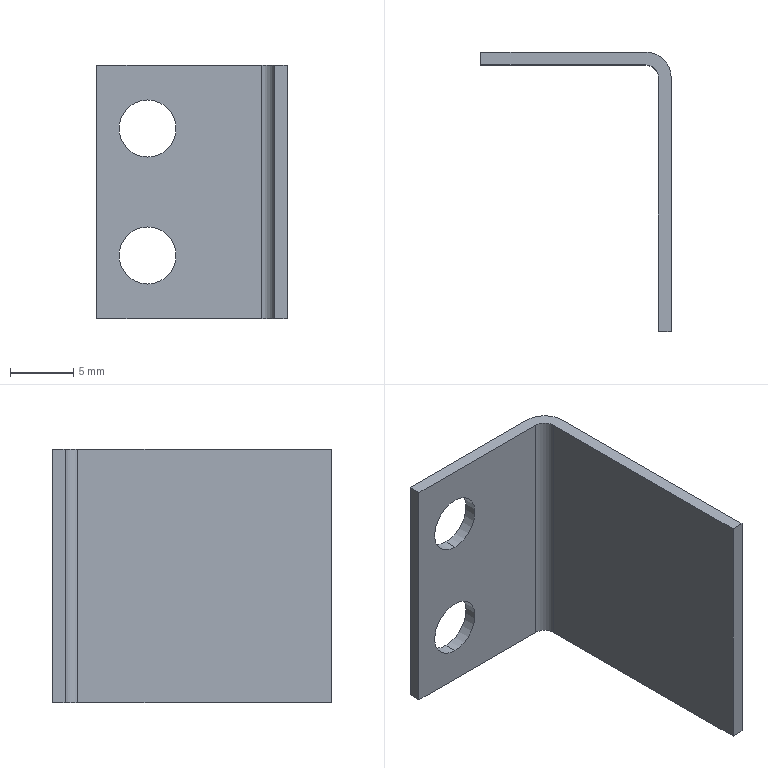Part | STEP file | 0243_222_Dog | 1 solid | 14 faces | box 15 x 22 x 20 mm | volume 675.315 mm3 | plane 8 | cylinder 6 | commonest cylinder face diameters 4.5 x4 2 x1 4 x1
STEP:
#1=CARTESIAN_POINT('',(0.,0.,0.));
#2=DIRECTION('',(0.,0.,1.));
#3=DIRECTION('',(1.,0.,0.));
#4=AXIS2_PLACEMENT_3D('',#1,#2,#3);
#5=CARTESIAN_POINT('',(-11.,-1.,7.25));
#6=VERTEX_POINT('',#5);
#7=CARTESIAN_POINT('',(-11.,0.,7.25));
#8=VERTEX_POINT('',#7);
#9=CARTESIAN_POINT('',(-11.,0.,7.25));
#10=DIRECTION('',(0.,1.,0.));
#11=VECTOR('',#10,1.);
#12=LINE('',#9,#11);
#13=CARTESIAN_POINT('',(-11.,0.,5.));
#14=DIRECTION('',(0.,1.,0.));
#15=DIRECTION('',(0.,0.,1.));
#16=AXIS2_PLACEMENT_3D('',#13,#14,#15);
#17=CYLINDRICAL_SURFACE('',#16,2.25);
#18=CARTESIAN_POINT('',(6.283,0.));
#19=DIRECTION('',(0.,1.));
#20=VECTOR('',#19,1.);
#21=LINE('',#18,#20);
#22=(GEOMETRIC_REPRESENTATION_CONTEXT(2)PARAMETRIC_REPRESENTATION_CONTEXT()REPRESENTATION_CONTEXT('',''));
#23=DEFINITIONAL_REPRESENTATION('',(#21),#22);
#24=PCURVE('',#17,#23);
#25=CARTESIAN_POINT('',(-11.,0.,5.));
#26=DIRECTION('',(0.,1.,0.));
#27=DIRECTION('',(0.,0.,1.));
#28=AXIS2_PLACEMENT_3D('',#25,#26,#27);
#29=CYLINDRICAL_SURFACE('',#28,2.25);
#30=CARTESIAN_POINT('',(0.,0.));
#31=DIRECTION('',(0.,1.));
#32=VECTOR('',#31,1.);
#33=LINE('',#30,#32);
#34=(GEOMETRIC_REPRESENTATION_CONTEXT(2)PARAMETRIC_REPRESENTATION_CONTEXT()REPRESENTATION_CONTEXT('',''));
#35=DEFINITIONAL_REPRESENTATION('',(#33),#34);
#36=PCURVE('',#29,#35);
#37=SURFACE_CURVE('',#12,(#24,#36),.PCURVE_S1.);
#38=EDGE_CURVE('',#6,#8,#37,.T.);
#39=ORIENTED_EDGE('',*,*,#38,.T.);
#40=CARTESIAN_POINT('',(-11.,0.,2.75));
#41=VERTEX_POINT('',#40);
#42=CARTESIAN_POINT('',(-11.,0.,5.));
#43=DIRECTION('',(0.,1.,0.));
#44=DIRECTION('',(0.,0.,1.));
#45=AXIS2_PLACEMENT_3D('',#42,#43,#44);
#46=CIRCLE('',#45,2.25);
#47=CARTESIAN_POINT('',(0.,0.));
#48=DIRECTION('',(1.,0.));
#49=VECTOR('',#48,1.);
#50=LINE('',#47,#49);
#51=(GEOMETRIC_REPRESENTATION_CONTEXT(2)PARAMETRIC_REPRESENTATION_CONTEXT()REPRESENTATION_CONTEXT('',''));
#52=DEFINITIONAL_REPRESENTATION('',(#50),#51);
#53=PCURVE('',#17,#52);
#54=CARTESIAN_POINT('',(-15.,0.,10.));
#55=DIRECTION('',(0.,-1.,0.));
#56=DIRECTION('',(0.,0.,-1.));
#57=AXIS2_PLACEMENT_3D('',#54,#55,#56);
#58=PLANE('',#57);
#59=CARTESIAN_POINT('',(2.75,4.));
#60=CARTESIAN_POINT('',(2.75,7.897));
#61=CARTESIAN_POINT('',(6.125,5.949));
#62=CARTESIAN_POINT('',(9.5,4.));
#63=CARTESIAN_POINT('',(6.125,2.051));
#64=CARTESIAN_POINT('',(2.75,0.1029));
#65=CARTESIAN_POINT('',(2.75,4.));
#66=(BOUNDED_CURVE()B_SPLINE_CURVE(2,(#59,#60,#61,#62,#63,#64,#65),.UNSPECIFIED.,.T.,.F.)B_SPLINE_CURVE_WITH_KNOTS((1,2,2,2,2,1),(-2.094,0.,2.094,4.189,6.283,8.378),.UNSPECIFIED.)CURVE()GEOMETRIC_REPRESENTATION_ITEM()RATIONAL_B_SPLINE_CURVE((1.,0.5,1.,0.5,1.,0.5,1.))REPRESENTATION_ITEM(''));
#67=(GEOMETRIC_REPRESENTATION_CONTEXT(2)PARAMETRIC_REPRESENTATION_CONTEXT()REPRESENTATION_CONTEXT('',''));
#68=DEFINITIONAL_REPRESENTATION('',(#66),#67);
#69=PCURVE('',#58,#68);
#70=SURFACE_CURVE('',#46,(#53,#69),.PCURVE_S1.);
#71=EDGE_CURVE('',#41,#8,#70,.T.);
#72=ORIENTED_EDGE('',*,*,#71,.F.);
#73=CARTESIAN_POINT('',(-11.,-1.,2.75));
#74=VERTEX_POINT('',#73);
#75=CARTESIAN_POINT('',(-11.,0.,2.75));
#76=DIRECTION('',(0.,1.,0.));
#77=VECTOR('',#76,1.);
#78=LINE('',#75,#77);
#79=CARTESIAN_POINT('',(3.142,0.));
#80=DIRECTION('',(0.,1.));
#81=VECTOR('',#80,1.);
#82=LINE('',#79,#81);
#83=(GEOMETRIC_REPRESENTATION_CONTEXT(2)PARAMETRIC_REPRESENTATION_CONTEXT()REPRESENTATION_CONTEXT('',''));
#84=DEFINITIONAL_REPRESENTATION('',(#82),#83);
#85=PCURVE('',#17,#84);
#86=CARTESIAN_POINT('',(3.142,0.));
#87=DIRECTION('',(0.,1.));
#88=VECTOR('',#87,1.);
#89=LINE('',#86,#88);
#90=(GEOMETRIC_REPRESENTATION_CONTEXT(2)PARAMETRIC_REPRESENTATION_CONTEXT()REPRESENTATION_CONTEXT('',''));
#91=DEFINITIONAL_REPRESENTATION('',(#89),#90);
#92=PCURVE('',#29,#91);
#93=SURFACE_CURVE('',#78,(#85,#92),.PCURVE_S1.);
#94=EDGE_CURVE('',#74,#41,#93,.T.);
#95=ORIENTED_EDGE('',*,*,#94,.F.);
#96=CARTESIAN_POINT('',(-11.,-1.,5.));
#97=DIRECTION('',(0.,1.,0.));
#98=DIRECTION('',(-1.,0.,0.));
#99=AXIS2_PLACEMENT_3D('',#96,#97,#98);
#100=CIRCLE('',#99,2.25);
#101=CARTESIAN_POINT('',(-1.571,-1.));
#102=DIRECTION('',(1.,0.));
#103=VECTOR('',#102,1.);
#104=LINE('',#101,#103);
#105=(GEOMETRIC_REPRESENTATION_CONTEXT(2)PARAMETRIC_REPRESENTATION_CONTEXT()REPRESENTATION_CONTEXT('',''));
#106=DEFINITIONAL_REPRESENTATION('',(#104),#105);
#107=PCURVE('',#17,#106);
#108=CARTESIAN_POINT('',(-15.,-1.,10.));
#109=DIRECTION('',(0.,1.,0.));
#110=DIRECTION('',(-1.,0.,0.));
#111=AXIS2_PLACEMENT_3D('',#108,#109,#110);
#112=PLANE('',#111);
#113=CARTESIAN_POINT('',(-4.,-5.));
#114=DIRECTION('',(1.,0.));
#115=AXIS2_PLACEMENT_2D('',#113,#114);
#116=CIRCLE('',#115,2.25);
#117=(GEOMETRIC_REPRESENTATION_CONTEXT(2)PARAMETRIC_REPRESENTATION_CONTEXT()REPRESENTATION_CONTEXT('',''));
#118=DEFINITIONAL_REPRESENTATION('',(#116),#117);
#119=PCURVE('',#112,#118);
#120=SURFACE_CURVE('',#100,(#107,#119),.PCURVE_S1.);
#121=EDGE_CURVE('',#74,#6,#120,.T.);
#122=ORIENTED_EDGE('',*,*,#121,.T.);
#123=EDGE_LOOP('',(#39,#72,#95,#122));
#124=FACE_BOUND('',#123,.F.);
#125=ADVANCED_FACE('',(#124),#17,.F.);
#126=CARTESIAN_POINT('',(-11.,-1.,-2.75));
#127=VERTEX_POINT('',#126);
#128=CARTESIAN_POINT('',(-11.,0.,-2.75));
#129=VERTEX_POINT('',#128);
#130=CARTESIAN_POINT('',(-11.,0.,-2.75));
#131=DIRECTION('',(0.,1.,0.));
#132=VECTOR('',#131,1.);
#133=LINE('',#130,#132);
#134=CARTESIAN_POINT('',(-11.,0.,-5.));
#135=DIRECTION('',(0.,1.,0.));
#136=DIRECTION('',(0.,0.,1.));
#137=AXIS2_PLACEMENT_3D('',#134,#135,#136);
#138=CYLINDRICAL_SURFACE('',#137,2.25);
#139=CARTESIAN_POINT('',(6.283,0.));
#140=DIRECTION('',(0.,1.));
#141=VECTOR('',#140,1.);
#142=LINE('',#139,#141);
#143=(GEOMETRIC_REPRESENTATION_CONTEXT(2)PARAMETRIC_REPRESENTATION_CONTEXT()REPRESENTATION_CONTEXT('',''));
#144=DEFINITIONAL_REPRESENTATION('',(#142),#143);
#145=PCURVE('',#138,#144);
#146=CARTESIAN_POINT('',(-11.,0.,-5.));
#147=DIRECTION('',(0.,1.,0.));
#148=DIRECTION('',(0.,0.,1.));
#149=AXIS2_PLACEMENT_3D('',#146,#147,#148);
#150=CYLINDRICAL_SURFACE('',#149,2.25);
#151=CARTESIAN_POINT('',(0.,0.));
#152=DIRECTION('',(0.,1.));
#153=VECTOR('',#152,1.);
#154=LINE('',#151,#153);
#155=(GEOMETRIC_REPRESENTATION_CONTEXT(2)PARAMETRIC_REPRESENTATION_CONTEXT()REPRESENTATION_CONTEXT('',''));
#156=DEFINITIONAL_REPRESENTATION('',(#154),#155);
#157=PCURVE('',#150,#156);
#158=SURFACE_CURVE('',#133,(#145,#157),.PCURVE_S1.);
#159=EDGE_CURVE('',#127,#129,#158,.T.);
#160=ORIENTED_EDGE('',*,*,#159,.T.);
#161=CARTESIAN_POINT('',(-11.,0.,-7.25));
#162=VERTEX_POINT('',#161);
#163=CARTESIAN_POINT('',(-11.,0.,-5.));
#164=DIRECTION('',(0.,1.,0.));
#165=DIRECTION('',(0.,0.,1.));
#166=AXIS2_PLACEMENT_3D('',#163,#164,#165);
#167=CIRCLE('',#166,2.25);
#168=CARTESIAN_POINT('',(0.,0.));
#169=DIRECTION('',(1.,0.));
#170=VECTOR('',#169,1.);
#171=LINE('',#168,#170);
#172=(GEOMETRIC_REPRESENTATION_CONTEXT(2)PARAMETRIC_REPRESENTATION_CONTEXT()REPRESENTATION_CONTEXT('',''));
#173=DEFINITIONAL_REPRESENTATION('',(#171),#172);
#174=PCURVE('',#138,#173);
#175=CARTESIAN_POINT('',(12.75,4.));
#176=CARTESIAN_POINT('',(12.75,7.897));
#177=CARTESIAN_POINT('',(16.125,5.949));
#178=CARTESIAN_POINT('',(19.5,4.));
#179=CARTESIAN_POINT('',(16.125,2.051));
#180=CARTESIAN_POINT('',(12.75,0.1029));
#181=CARTESIAN_POINT('',(12.75,4.));
#182=(BOUNDED_CURVE()B_SPLINE_CURVE(2,(#175,#176,#177,#178,#179,#180,#181),.UNSPECIFIED.,.T.,.F.)B_SPLINE_CURVE_WITH_KNOTS((1,2,2,2,2,1),(-2.094,0.,2.094,4.189,6.283,8.378),.UNSPECIFIED.)CURVE()GEOMETRIC_REPRESENTATION_ITEM()RATIONAL_B_SPLINE_CURVE((1.,0.5,1.,0.5,1.,0.5,1.))REPRESENTATION_ITEM(''));
#183=(GEOMETRIC_REPRESENTATION_CONTEXT(2)PARAMETRIC_REPRESENTATION_CONTEXT()REPRESENTATION_CONTEXT('',''));
#184=DEFINITIONAL_REPRESENTATION('',(#182),#183);
#185=PCURVE('',#58,#184);
#186=SURFACE_CURVE('',#167,(#174,#185),.PCURVE_S1.);
#187=EDGE_CURVE('',#162,#129,#186,.T.);
#188=ORIENTED_EDGE('',*,*,#187,.F.);
#189=CARTESIAN_POINT('',(-11.,-1.,-7.25));
#190=VERTEX_POINT('',#189);
#191=CARTESIAN_POINT('',(-11.,0.,-7.25));
#192=DIRECTION('',(0.,1.,0.));
#193=VECTOR('',#192,1.);
#194=LINE('',#191,#193);
#195=CARTESIAN_POINT('',(3.142,0.));
#196=DIRECTION('',(0.,1.));
#197=VECTOR('',#196,1.);
#198=LINE('',#195,#197);
#199=(GEOMETRIC_REPRESENTATION_CONTEXT(2)PARAMETRIC_REPRESENTATION_CONTEXT()REPRESENTATION_CONTEXT('',''));
#200=DEFINITIONAL_REPRESENTATION('',(#198),#199);
#201=PCURVE('',#138,#200);
#202=CARTESIAN_POINT('',(3.142,0.));
#203=DIRECTION('',(0.,1.));
#204=VECTOR('',#203,1.);
#205=LINE('',#202,#204);
#206=(GEOMETRIC_REPRESENTATION_CONTEXT(2)PARAMETRIC_REPRESENTATION_CONTEXT()REPRESENTATION_CONTEXT('',''));
#207=DEFINITIONAL_REPRESENTATION('',(#205),#206);
#208=PCURVE('',#150,#207);
#209=SURFACE_CURVE('',#194,(#201,#208),.PCURVE_S1.);
#210=EDGE_CURVE('',#190,#162,#209,.T.);
#211=ORIENTED_EDGE('',*,*,#210,.F.);
#212=CARTESIAN_POINT('',(-11.,-1.,-5.));
#213=DIRECTION('',(0.,1.,0.));
#214=DIRECTION('',(-1.,0.,0.));
#215=AXIS2_PLACEMENT_3D('',#212,#213,#214);
#216=CIRCLE('',#215,2.25);
#217=CARTESIAN_POINT('',(-1.571,-1.));
#218=DIRECTION('',(1.,0.));
#219=VECTOR('',#218,1.);
#220=LINE('',#217,#219);
#221=(GEOMETRIC_REPRESENTATION_CONTEXT(2)PARAMETRIC_REPRESENTATION_CONTEXT()REPRESENTATION_CONTEXT('',''));
#222=DEFINITIONAL_REPRESENTATION('',(#220),#221);
#223=PCURVE('',#138,#222);
#224=CARTESIAN_POINT('',(-4.,-15.));
#225=DIRECTION('',(1.,0.));
#226=AXIS2_PLACEMENT_2D('',#224,#225);
#227=CIRCLE('',#226,2.25);
#228=(GEOMETRIC_REPRESENTATION_CONTEXT(2)PARAMETRIC_REPRESENTATION_CONTEXT()REPRESENTATION_CONTEXT('',''));
#229=DEFINITIONAL_REPRESENTATION('',(#227),#228);
#230=PCURVE('',#112,#229);
#231=SURFACE_CURVE('',#216,(#223,#230),.PCURVE_S1.);
#232=EDGE_CURVE('',#190,#127,#231,.T.);
#233=ORIENTED_EDGE('',*,*,#232,.T.);
#234=EDGE_LOOP('',(#160,#188,#211,#233));
#235=FACE_BOUND('',#234,.F.);
#236=ADVANCED_FACE('',(#235),#138,.F.);
#237=CARTESIAN_POINT('',(-15.,0.,-10.));
#238=VERTEX_POINT('',#237);
#239=CARTESIAN_POINT('',(-15.,-1.,-10.));
#240=VERTEX_POINT('',#239);
#241=CARTESIAN_POINT('',(-15.,0.,-10.));
#242=DIRECTION('',(0.,-1.,0.));
#243=VECTOR('',#242,1.);
#244=LINE('',#241,#243);
#245=CARTESIAN_POINT('',(-15.,0.,10.));
#246=DIRECTION('',(1.,0.,0.));
#247=DIRECTION('',(0.,0.,-1.));
#248=AXIS2_PLACEMENT_3D('',#245,#246,#247);
#249=PLANE('',#248);
#250=CARTESIAN_POINT('',(20.,0.));
#251=DIRECTION('',(0.,-1.));
#252=VECTOR('',#251,1.);
#253=LINE('',#250,#252);
#254=(GEOMETRIC_REPRESENTATION_CONTEXT(2)PARAMETRIC_REPRESENTATION_CONTEXT()REPRESENTATION_CONTEXT('',''));
#255=DEFINITIONAL_REPRESENTATION('',(#253),#254);
#256=PCURVE('',#249,#255);
#257=CARTESIAN_POINT('',(-15.,-1.,-10.));
#258=DIRECTION('',(0.,0.,1.));
#259=DIRECTION('',(1.,0.,0.));
#260=AXIS2_PLACEMENT_3D('',#257,#258,#259);
#261=PLANE('',#260);
#262=CARTESIAN_POINT('',(0.,1.));
#263=DIRECTION('',(0.,-1.));
#264=VECTOR('',#263,1.);
#265=LINE('',#262,#264);
#266=(GEOMETRIC_REPRESENTATION_CONTEXT(2)PARAMETRIC_REPRESENTATION_CONTEXT()REPRESENTATION_CONTEXT('',''));
#267=DEFINITIONAL_REPRESENTATION('',(#265),#266);
#268=PCURVE('',#261,#267);
#269=SURFACE_CURVE('',#244,(#256,#268),.PCURVE_S1.);
#270=EDGE_CURVE('',#238,#240,#269,.T.);
#271=ORIENTED_EDGE('',*,*,#270,.T.);
#272=CARTESIAN_POINT('',(-15.,-1.,10.));
#273=VERTEX_POINT('',#272);
#274=CARTESIAN_POINT('',(-15.,-1.,10.));
#275=DIRECTION('',(0.,0.,-1.));
#276=VECTOR('',#275,1.);
#277=LINE('',#274,#276);
#278=CARTESIAN_POINT('',(0.,-1.));
#279=DIRECTION('',(1.,0.));
#280=VECTOR('',#279,1.);
#281=LINE('',#278,#280);
#282=(GEOMETRIC_REPRESENTATION_CONTEXT(2)PARAMETRIC_REPRESENTATION_CONTEXT()REPRESENTATION_CONTEXT('',''));
#283=DEFINITIONAL_REPRESENTATION('',(#281),#282);
#284=PCURVE('',#249,#283);
#285=CARTESIAN_POINT('',(0.,0.));
#286=DIRECTION('',(0.,-1.));
#287=VECTOR('',#286,1.);
#288=LINE('',#285,#287);
#289=(GEOMETRIC_REPRESENTATION_CONTEXT(2)PARAMETRIC_REPRESENTATION_CONTEXT()REPRESENTATION_CONTEXT('',''));
#290=DEFINITIONAL_REPRESENTATION('',(#288),#289);
#291=PCURVE('',#112,#290);
#292=SURFACE_CURVE('',#277,(#284,#291),.PCURVE_S1.);
#293=EDGE_CURVE('',#273,#240,#292,.T.);
#294=ORIENTED_EDGE('',*,*,#293,.F.);
#295=CARTESIAN_POINT('',(-15.,0.,10.));
#296=VERTEX_POINT('',#295);
#297=CARTESIAN_POINT('',(-15.,0.,10.));
#298=DIRECTION('',(0.,-1.,0.));
#299=VECTOR('',#298,1.);
#300=LINE('',#297,#299);
#301=CARTESIAN_POINT('',(0.,0.));
#302=DIRECTION('',(0.,-1.));
#303=VECTOR('',#302,1.);
#304=LINE('',#301,#303);
#305=(GEOMETRIC_REPRESENTATION_CONTEXT(2)PARAMETRIC_REPRESENTATION_CONTEXT()REPRESENTATION_CONTEXT('',''));
#306=DEFINITIONAL_REPRESENTATION('',(#304),#305);
#307=PCURVE('',#249,#306);
#308=CARTESIAN_POINT('',(-15.,-1.,10.));
#309=DIRECTION('',(0.,0.,1.));
#310=DIRECTION('',(1.,0.,0.));
#311=AXIS2_PLACEMENT_3D('',#308,#309,#310);
#312=PLANE('',#311);
#313=CARTESIAN_POINT('',(0.,1.));
#314=DIRECTION('',(0.,-1.));
#315=VECTOR('',#314,1.);
#316=LINE('',#313,#315);
#317=(GEOMETRIC_REPRESENTATION_CONTEXT(2)PARAMETRIC_REPRESENTATION_CONTEXT()REPRESENTATION_CONTEXT('',''));
#318=DEFINITIONAL_REPRESENTATION('',(#316),#317);
#319=PCURVE('',#312,#318);
#320=SURFACE_CURVE('',#300,(#307,#319),.PCURVE_S1.);
#321=EDGE_CURVE('',#296,#273,#320,.T.);
#322=ORIENTED_EDGE('',*,*,#321,.F.);
#323=CARTESIAN_POINT('',(-15.,0.,10.));
#324=DIRECTION('',(0.,0.,-1.));
#325=VECTOR('',#324,1.);
#326=LINE('',#323,#325);
#327=CARTESIAN_POINT('',(0.,0.));
#328=DIRECTION('',(1.,0.));
#329=VECTOR('',#328,1.);
#330=LINE('',#327,#329);
#331=(GEOMETRIC_REPRESENTATION_CONTEXT(2)PARAMETRIC_REPRESENTATION_CONTEXT()REPRESENTATION_CONTEXT('',''));
#332=DEFINITIONAL_REPRESENTATION('',(#330),#331);
#333=PCURVE('',#249,#332);
#334=CARTESIAN_POINT('',(0.,0.));
#335=DIRECTION('',(1.,0.));
#336=VECTOR('',#335,1.);
#337=LINE('',#334,#336);
#338=(GEOMETRIC_REPRESENTATION_CONTEXT(2)PARAMETRIC_REPRESENTATION_CONTEXT()REPRESENTATION_CONTEXT('',''));
#339=DEFINITIONAL_REPRESENTATION('',(#337),#338);
#340=PCURVE('',#58,#339);
#341=SURFACE_CURVE('',#326,(#333,#340),.PCURVE_S1.);
#342=EDGE_CURVE('',#296,#238,#341,.T.);
#343=ORIENTED_EDGE('',*,*,#342,.T.);
#344=EDGE_LOOP('',(#271,#294,#322,#343));
#345=FACE_BOUND('',#344,.T.);
#346=ADVANCED_FACE('',(#345),#249,.F.);
#347=CARTESIAN_POINT('',(-11.,-1.,5.));
#348=DIRECTION('',(0.,1.,0.));
#349=DIRECTION('',(-1.,0.,0.));
#350=AXIS2_PLACEMENT_3D('',#347,#348,#349);
#351=CIRCLE('',#350,2.25);
#352=CARTESIAN_POINT('',(-4.,-5.));
#353=DIRECTION('',(1.,0.));
#354=AXIS2_PLACEMENT_2D('',#352,#353);
#355=CIRCLE('',#354,2.25);
#356=(GEOMETRIC_REPRESENTATION_CONTEXT(2)PARAMETRIC_REPRESENTATION_CONTEXT()REPRESENTATION_CONTEXT('',''));
#357=DEFINITIONAL_REPRESENTATION('',(#355),#356);
#358=PCURVE('',#112,#357);
#359=CARTESIAN_POINT('',(-1.571,-1.));
#360=DIRECTION('',(1.,0.));
#361=VECTOR('',#360,1.);
#362=LINE('',#359,#361);
#363=(GEOMETRIC_REPRESENTATION_CONTEXT(2)PARAMETRIC_REPRESENTATION_CONTEXT()REPRESENTATION_CONTEXT('',''));
#364=DEFINITIONAL_REPRESENTATION('',(#362),#363);
#365=PCURVE('',#29,#364);
#366=SURFACE_CURVE('',#351,(#358,#365),.PCURVE_S1.);
#367=EDGE_CURVE('',#6,#74,#366,.T.);
#368=ORIENTED_EDGE('',*,*,#367,.T.);
#369=ORIENTED_EDGE('',*,*,#121,.T.);
#370=EDGE_LOOP('',(#368,#369));
#371=FACE_BOUND('',#370,.T.);
#372=CARTESIAN_POINT('',(-11.,-1.,-5.));
#373=DIRECTION('',(0.,1.,0.));
#374=DIRECTION('',(-1.,0.,0.));
#375=AXIS2_PLACEMENT_3D('',#372,#373,#374);
#376=CIRCLE('',#375,2.25);
#377=CARTESIAN_POINT('',(-4.,-15.));
#378=DIRECTION('',(1.,0.));
#379=AXIS2_PLACEMENT_2D('',#377,#378);
#380=CIRCLE('',#379,2.25);
#381=(GEOMETRIC_REPRESENTATION_CONTEXT(2)PARAMETRIC_REPRESENTATION_CONTEXT()REPRESENTATION_CONTEXT('',''));
#382=DEFINITIONAL_REPRESENTATION('',(#380),#381);
#383=PCURVE('',#112,#382);
#384=CARTESIAN_POINT('',(-1.571,-1.));
#385=DIRECTION('',(1.,0.));
#386=VECTOR('',#385,1.);
#387=LINE('',#384,#386);
#388=(GEOMETRIC_REPRESENTATION_CONTEXT(2)PARAMETRIC_REPRESENTATION_CONTEXT()REPRESENTATION_CONTEXT('',''));
#389=DEFINITIONAL_REPRESENTATION('',(#387),#388);
#390=PCURVE('',#150,#389);
#391=SURFACE_CURVE('',#376,(#383,#390),.PCURVE_S1.);
#392=EDGE_CURVE('',#127,#190,#391,.T.);
#393=ORIENTED_EDGE('',*,*,#392,.T.);
#394=ORIENTED_EDGE('',*,*,#232,.T.);
#395=EDGE_LOOP('',(#393,#394));
#396=FACE_BOUND('',#395,.T.);
#397=CARTESIAN_POINT('',(-2.,-1.,-10.));
#398=VERTEX_POINT('',#397);
#399=CARTESIAN_POINT('',(-15.,-1.,-10.));
#400=DIRECTION('',(1.,0.,0.));
#401=VECTOR('',#400,1.);
#402=LINE('',#399,#401);
#403=CARTESIAN_POINT('',(0.,-20.));
#404=DIRECTION('',(-1.,0.));
#405=VECTOR('',#404,1.);
#406=LINE('',#403,#405);
#407=(GEOMETRIC_REPRESENTATION_CONTEXT(2)PARAMETRIC_REPRESENTATION_CONTEXT()REPRESENTATION_CONTEXT('',''));
#408=DEFINITIONAL_REPRESENTATION('',(#406),#407);
#409=PCURVE('',#112,#408);
#410=CARTESIAN_POINT('',(0.,0.));
#411=DIRECTION('',(1.,0.));
#412=VECTOR('',#411,1.);
#413=LINE('',#410,#412);
#414=(GEOMETRIC_REPRESENTATION_CONTEXT(2)PARAMETRIC_REPRESENTATION_CONTEXT()REPRESENTATION_CONTEXT('',''));
#415=DEFINITIONAL_REPRESENTATION('',(#413),#414);
#416=PCURVE('',#261,#415);
#417=SURFACE_CURVE('',#402,(#409,#416),.PCURVE_S1.);
#418=EDGE_CURVE('',#240,#398,#417,.T.);
#419=ORIENTED_EDGE('',*,*,#418,.T.);
#420=CARTESIAN_POINT('',(-2.,-1.,10.));
#421=VERTEX_POINT('',#420);
#422=CARTESIAN_POINT('',(-2.,-1.,10.));
#423=DIRECTION('',(0.,0.,1.));
#424=VECTOR('',#423,1.);
#425=LINE('',#422,#424);
#426=CARTESIAN_POINT('',(-13.,0.));
#427=DIRECTION('',(0.,1.));
#428=VECTOR('',#427,1.);
#429=LINE('',#426,#428);
#430=(GEOMETRIC_REPRESENTATION_CONTEXT(2)PARAMETRIC_REPRESENTATION_CONTEXT()REPRESENTATION_CONTEXT('',''));
#431=DEFINITIONAL_REPRESENTATION('',(#429),#430);
#432=PCURVE('',#112,#431);
#433=CARTESIAN_POINT('',(-2.,-2.,10.));
#434=DIRECTION('',(0.,0.,1.));
#435=DIRECTION('',(1.,0.,0.));
#436=AXIS2_PLACEMENT_3D('',#433,#434,#435);
#437=CYLINDRICAL_SURFACE('',#436,1.);
#438=CARTESIAN_POINT('',(1.571,0.));
#439=DIRECTION('',(0.,1.));
#440=VECTOR('',#439,1.);
#441=LINE('',#438,#440);
#442=(GEOMETRIC_REPRESENTATION_CONTEXT(2)PARAMETRIC_REPRESENTATION_CONTEXT()REPRESENTATION_CONTEXT('',''));
#443=DEFINITIONAL_REPRESENTATION('',(#441),#442);
#444=PCURVE('',#437,#443);
#445=SURFACE_CURVE('',#425,(#432,#444),.PCURVE_S1.);
#446=EDGE_CURVE('',#398,#421,#445,.T.);
#447=ORIENTED_EDGE('',*,*,#446,.T.);
#448=CARTESIAN_POINT('',(-15.,-1.,10.));
#449=DIRECTION('',(1.,0.,0.));
#450=VECTOR('',#449,1.);
#451=LINE('',#448,#450);
#452=CARTESIAN_POINT('',(0.,0.));
#453=DIRECTION('',(-1.,0.));
#454=VECTOR('',#453,1.);
#455=LINE('',#452,#454);
#456=(GEOMETRIC_REPRESENTATION_CONTEXT(2)PARAMETRIC_REPRESENTATION_CONTEXT()REPRESENTATION_CONTEXT('',''));
#457=DEFINITIONAL_REPRESENTATION('',(#455),#456);
#458=PCURVE('',#112,#457);
#459=CARTESIAN_POINT('',(0.,0.));
#460=DIRECTION('',(1.,0.));
#461=VECTOR('',#460,1.);
#462=LINE('',#459,#461);
#463=(GEOMETRIC_REPRESENTATION_CONTEXT(2)PARAMETRIC_REPRESENTATION_CONTEXT()REPRESENTATION_CONTEXT('',''));
#464=DEFINITIONAL_REPRESENTATION('',(#462),#463);
#465=PCURVE('',#312,#464);
#466=SURFACE_CURVE('',#451,(#458,#465),.PCURVE_S1.);
#467=EDGE_CURVE('',#273,#421,#466,.T.);
#468=ORIENTED_EDGE('',*,*,#467,.F.);
#469=ORIENTED_EDGE('',*,*,#293,.T.);
#470=EDGE_LOOP('',(#419,#447,#468,#469));
#471=FACE_BOUND('',#470,.T.);
#472=ADVANCED_FACE('',(#371,#396,#471),#112,.F.);
#473=CARTESIAN_POINT('',(-1.,-2.,10.));
#474=VERTEX_POINT('',#473);
#475=CARTESIAN_POINT('',(-1.,-22.,10.));
#476=VERTEX_POINT('',#475);
#477=CARTESIAN_POINT('',(-1.,-1.,10.));
#478=DIRECTION('',(0.,-1.,0.));
#479=VECTOR('',#478,1.);
#480=LINE('',#477,#479);
#481=CARTESIAN_POINT('',(-1.,-1.,10.));
#482=DIRECTION('',(1.,0.,0.));
#483=DIRECTION('',(0.,1.,0.));
#484=AXIS2_PLACEMENT_3D('',#481,#482,#483);
#485=PLANE('',#484);
#486=CARTESIAN_POINT('',(0.,0.));
#487=DIRECTION('',(-1.,0.));
#488=VECTOR('',#487,1.);
#489=LINE('',#486,#488);
#490=(GEOMETRIC_REPRESENTATION_CONTEXT(2)PARAMETRIC_REPRESENTATION_CONTEXT()REPRESENTATION_CONTEXT('',''));
#491=DEFINITIONAL_REPRESENTATION('',(#489),#490);
#492=PCURVE('',#485,#491);
#493=CARTESIAN_POINT('',(14.,0.));
#494=DIRECTION('',(0.,-1.));
#495=VECTOR('',#494,1.);
#496=LINE('',#493,#495);
#497=(GEOMETRIC_REPRESENTATION_CONTEXT(2)PARAMETRIC_REPRESENTATION_CONTEXT()REPRESENTATION_CONTEXT('',''));
#498=DEFINITIONAL_REPRESENTATION('',(#496),#497);
#499=PCURVE('',#312,#498);
#500=SURFACE_CURVE('',#480,(#492,#499),.PCURVE_S1.);
#501=EDGE_CURVE('',#474,#476,#500,.T.);
#502=ORIENTED_EDGE('',*,*,#501,.F.);
#503=CARTESIAN_POINT('',(-1.,-2.,-10.));
#504=VERTEX_POINT('',#503);
#505=CARTESIAN_POINT('',(-1.,-2.,-10.));
#506=DIRECTION('',(0.,0.,-1.));
#507=VECTOR('',#506,1.);
#508=LINE('',#505,#507);
#509=CARTESIAN_POINT('',(-1.,-20.));
#510=DIRECTION('',(0.,-1.));
#511=VECTOR('',#510,1.);
#512=LINE('',#509,#511);
#513=(GEOMETRIC_REPRESENTATION_CONTEXT(2)PARAMETRIC_REPRESENTATION_CONTEXT()REPRESENTATION_CONTEXT('',''));
#514=DEFINITIONAL_REPRESENTATION('',(#512),#513);
#515=PCURVE('',#485,#514);
#516=CARTESIAN_POINT('',(0.,-20.));
#517=DIRECTION('',(0.,-1.));
#518=VECTOR('',#517,1.);
#519=LINE('',#516,#518);
#520=(GEOMETRIC_REPRESENTATION_CONTEXT(2)PARAMETRIC_REPRESENTATION_CONTEXT()REPRESENTATION_CONTEXT('',''));
#521=DEFINITIONAL_REPRESENTATION('',(#519),#520);
#522=PCURVE('',#437,#521);
#523=SURFACE_CURVE('',#508,(#515,#522),.PCURVE_S1.);
#524=EDGE_CURVE('',#474,#504,#523,.T.);
#525=ORIENTED_EDGE('',*,*,#524,.T.);
#526=CARTESIAN_POINT('',(-1.,-22.,-10.));
#527=VERTEX_POINT('',#526);
#528=CARTESIAN_POINT('',(-1.,-1.,-10.));
#529=DIRECTION('',(0.,-1.,0.));
#530=VECTOR('',#529,1.);
#531=LINE('',#528,#530);
#532=CARTESIAN_POINT('',(0.,-20.));
#533=DIRECTION('',(-1.,0.));
#534=VECTOR('',#533,1.);
#535=LINE('',#532,#534);
#536=(GEOMETRIC_REPRESENTATION_CONTEXT(2)PARAMETRIC_REPRESENTATION_CONTEXT()REPRESENTATION_CONTEXT('',''));
#537=DEFINITIONAL_REPRESENTATION('',(#535),#536);
#538=PCURVE('',#485,#537);
#539=CARTESIAN_POINT('',(14.,0.));
#540=DIRECTION('',(0.,-1.));
#541=VECTOR('',#540,1.);
#542=LINE('',#539,#541);
#543=(GEOMETRIC_REPRESENTATION_CONTEXT(2)PARAMETRIC_REPRESENTATION_CONTEXT()REPRESENTATION_CONTEXT('',''));
#544=DEFINITIONAL_REPRESENTATION('',(#542),#543);
#545=PCURVE('',#261,#544);
#546=SURFACE_CURVE('',#531,(#538,#545),.PCURVE_S1.);
#547=EDGE_CURVE('',#504,#527,#546,.T.);
#548=ORIENTED_EDGE('',*,*,#547,.T.);
#549=CARTESIAN_POINT('',(-1.,-22.,10.));
#550=DIRECTION('',(0.,0.,-1.));
#551=VECTOR('',#550,1.);
#552=LINE('',#549,#551);
#553=CARTESIAN_POINT('',(-21.,0.));
#554=DIRECTION('',(0.,-1.));
#555=VECTOR('',#554,1.);
#556=LINE('',#553,#555);
#557=(GEOMETRIC_REPRESENTATION_CONTEXT(2)PARAMETRIC_REPRESENTATION_CONTEXT()REPRESENTATION_CONTEXT('',''));
#558=DEFINITIONAL_REPRESENTATION('',(#556),#557);
#559=PCURVE('',#485,#558);
#560=CARTESIAN_POINT('',(0.,-22.,10.));
#561=DIRECTION('',(0.,1.,0.));
#562=DIRECTION('',(0.,0.,1.));
#563=AXIS2_PLACEMENT_3D('',#560,#561,#562);
#564=PLANE('',#563);
#565=CARTESIAN_POINT('',(0.,-1.));
#566=DIRECTION('',(-1.,0.));
#567=VECTOR('',#566,1.);
#568=LINE('',#565,#567);
#569=(GEOMETRIC_REPRESENTATION_CONTEXT(2)PARAMETRIC_REPRESENTATION_CONTEXT()REPRESENTATION_CONTEXT('',''));
#570=DEFINITIONAL_REPRESENTATION('',(#568),#569);
#571=PCURVE('',#564,#570);
#572=SURFACE_CURVE('',#552,(#559,#571),.PCURVE_S1.);
#573=EDGE_CURVE('',#476,#527,#572,.T.);
#574=ORIENTED_EDGE('',*,*,#573,.F.);
#575=EDGE_LOOP('',(#502,#525,#548,#574));
#576=FACE_BOUND('',#575,.T.);
#577=ADVANCED_FACE('',(#576),#485,.F.);
#578=CARTESIAN_POINT('',(0.,-22.,-10.));
#579=VERTEX_POINT('',#578);
#580=CARTESIAN_POINT('',(0.,-22.,-10.));
#581=DIRECTION('',(1.,0.,0.));
#582=VECTOR('',#581,1.);
#583=LINE('',#580,#582);
#584=CARTESIAN_POINT('',(-20.,0.));
#585=DIRECTION('',(0.,1.));
#586=VECTOR('',#585,1.);
#587=LINE('',#584,#586);
#588=(GEOMETRIC_REPRESENTATION_CONTEXT(2)PARAMETRIC_REPRESENTATION_CONTEXT()REPRESENTATION_CONTEXT('',''));
#589=DEFINITIONAL_REPRESENTATION('',(#587),#588);
#590=PCURVE('',#564,#589);
#591=CARTESIAN_POINT('',(15.,-21.));
#592=DIRECTION('',(1.,0.));
#593=VECTOR('',#592,1.);
#594=LINE('',#591,#593);
#595=(GEOMETRIC_REPRESENTATION_CONTEXT(2)PARAMETRIC_REPRESENTATION_CONTEXT()REPRESENTATION_CONTEXT('',''));
#596=DEFINITIONAL_REPRESENTATION('',(#594),#595);
#597=PCURVE('',#261,#596);
#598=SURFACE_CURVE('',#583,(#590,#597),.PCURVE_S1.);
#599=EDGE_CURVE('',#527,#579,#598,.T.);
#600=ORIENTED_EDGE('',*,*,#599,.T.);
#601=CARTESIAN_POINT('',(0.,-22.,10.));
#602=VERTEX_POINT('',#601);
#603=CARTESIAN_POINT('',(0.,-22.,10.));
#604=DIRECTION('',(0.,0.,-1.));
#605=VECTOR('',#604,1.);
#606=LINE('',#603,#605);
#607=CARTESIAN_POINT('',(0.,0.));
#608=DIRECTION('',(-1.,0.));
#609=VECTOR('',#608,1.);
#610=LINE('',#607,#609);
#611=(GEOMETRIC_REPRESENTATION_CONTEXT(2)PARAMETRIC_REPRESENTATION_CONTEXT()REPRESENTATION_CONTEXT('',''));
#612=DEFINITIONAL_REPRESENTATION('',(#610),#611);
#613=PCURVE('',#564,#612);
#614=CARTESIAN_POINT('',(0.,0.,10.));
#615=DIRECTION('',(-1.,0.,0.));
#616=DIRECTION('',(0.,-1.,0.));
#617=AXIS2_PLACEMENT_3D('',#614,#615,#616);
#618=PLANE('',#617);
#619=CARTESIAN_POINT('',(22.,0.));
#620=DIRECTION('',(0.,-1.));
#621=VECTOR('',#620,1.);
#622=LINE('',#619,#621);
#623=(GEOMETRIC_REPRESENTATION_CONTEXT(2)PARAMETRIC_REPRESENTATION_CONTEXT()REPRESENTATION_CONTEXT('',''));
#624=DEFINITIONAL_REPRESENTATION('',(#622),#623);
#625=PCURVE('',#618,#624);
#626=SURFACE_CURVE('',#606,(#613,#625),.PCURVE_S1.);
#627=EDGE_CURVE('',#602,#579,#626,.T.);
#628=ORIENTED_EDGE('',*,*,#627,.F.);
#629=CARTESIAN_POINT('',(0.,-22.,10.));
#630=DIRECTION('',(1.,0.,0.));
#631=VECTOR('',#630,1.);
#632=LINE('',#629,#631);
#633=CARTESIAN_POINT('',(0.,0.));
#634=DIRECTION('',(0.,1.));
#635=VECTOR('',#634,1.);
#636=LINE('',#633,#635);
#637=(GEOMETRIC_REPRESENTATION_CONTEXT(2)PARAMETRIC_REPRESENTATION_CONTEXT()REPRESENTATION_CONTEXT('',''));
#638=DEFINITIONAL_REPRESENTATION('',(#636),#637);
#639=PCURVE('',#564,#638);
#640=CARTESIAN_POINT('',(15.,-21.));
#641=DIRECTION('',(1.,0.));
#642=VECTOR('',#641,1.);
#643=LINE('',#640,#642);
#644=(GEOMETRIC_REPRESENTATION_CONTEXT(2)PARAMETRIC_REPRESENTATION_CONTEXT()REPRESENTATION_CONTEXT('',''));
#645=DEFINITIONAL_REPRESENTATION('',(#643),#644);
#646=PCURVE('',#312,#645);
#647=SURFACE_CURVE('',#632,(#639,#646),.PCURVE_S1.);
#648=EDGE_CURVE('',#476,#602,#647,.T.);
#649=ORIENTED_EDGE('',*,*,#648,.F.);
#650=ORIENTED_EDGE('',*,*,#573,.T.);
#651=EDGE_LOOP('',(#600,#628,#649,#650));
#652=FACE_BOUND('',#651,.T.);
#653=ADVANCED_FACE('',(#652),#564,.F.);
#654=CARTESIAN_POINT('',(0.,-2.,-10.));
#655=VERTEX_POINT('',#654);
#656=CARTESIAN_POINT('',(0.,0.,-10.));
#657=DIRECTION('',(0.,1.,0.));
#658=VECTOR('',#657,1.);
#659=LINE('',#656,#658);
#660=CARTESIAN_POINT('',(0.,-20.));
#661=DIRECTION('',(-1.,0.));
#662=VECTOR('',#661,1.);
#663=LINE('',#660,#662);
#664=(GEOMETRIC_REPRESENTATION_CONTEXT(2)PARAMETRIC_REPRESENTATION_CONTEXT()REPRESENTATION_CONTEXT('',''));
#665=DEFINITIONAL_REPRESENTATION('',(#663),#664);
#666=PCURVE('',#618,#665);
#667=CARTESIAN_POINT('',(15.,1.));
#668=DIRECTION('',(0.,1.));
#669=VECTOR('',#668,1.);
#670=LINE('',#667,#669);
#671=(GEOMETRIC_REPRESENTATION_CONTEXT(2)PARAMETRIC_REPRESENTATION_CONTEXT()REPRESENTATION_CONTEXT('',''));
#672=DEFINITIONAL_REPRESENTATION('',(#670),#671);
#673=PCURVE('',#261,#672);
#674=SURFACE_CURVE('',#659,(#666,#673),.PCURVE_S1.);
#675=EDGE_CURVE('',#579,#655,#674,.T.);
#676=ORIENTED_EDGE('',*,*,#675,.T.);
#677=CARTESIAN_POINT('',(0.,-2.,10.));
#678=VERTEX_POINT('',#677);
#679=CARTESIAN_POINT('',(0.,-2.,10.));
#680=DIRECTION('',(0.,0.,1.));
#681=VECTOR('',#680,1.);
#682=LINE('',#679,#681);
#683=CARTESIAN_POINT('',(2.,0.));
#684=DIRECTION('',(0.,1.));
#685=VECTOR('',#684,1.);
#686=LINE('',#683,#685);
#687=(GEOMETRIC_REPRESENTATION_CONTEXT(2)PARAMETRIC_REPRESENTATION_CONTEXT()REPRESENTATION_CONTEXT('',''));
#688=DEFINITIONAL_REPRESENTATION('',(#686),#687);
#689=PCURVE('',#618,#688);
#690=CARTESIAN_POINT('',(-2.,-2.,10.));
#691=DIRECTION('',(0.,0.,-1.));
#692=DIRECTION('',(-1.,0.,0.));
#693=AXIS2_PLACEMENT_3D('',#690,#691,#692);
#694=CYLINDRICAL_SURFACE('',#693,2.);
#695=CARTESIAN_POINT('',(3.142,0.));
#696=DIRECTION('',(0.,-1.));
#697=VECTOR('',#696,1.);
#698=LINE('',#695,#697);
#699=(GEOMETRIC_REPRESENTATION_CONTEXT(2)PARAMETRIC_REPRESENTATION_CONTEXT()REPRESENTATION_CONTEXT('',''));
#700=DEFINITIONAL_REPRESENTATION('',(#698),#699);
#701=PCURVE('',#694,#700);
#702=SURFACE_CURVE('',#682,(#689,#701),.PCURVE_S1.);
#703=EDGE_CURVE('',#655,#678,#702,.T.);
#704=ORIENTED_EDGE('',*,*,#703,.T.);
#705=CARTESIAN_POINT('',(0.,0.,10.));
#706=DIRECTION('',(0.,1.,0.));
#707=VECTOR('',#706,1.);
#708=LINE('',#705,#707);
#709=CARTESIAN_POINT('',(0.,0.));
#710=DIRECTION('',(-1.,0.));
#711=VECTOR('',#710,1.);
#712=LINE('',#709,#711);
#713=(GEOMETRIC_REPRESENTATION_CONTEXT(2)PARAMETRIC_REPRESENTATION_CONTEXT()REPRESENTATION_CONTEXT('',''));
#714=DEFINITIONAL_REPRESENTATION('',(#712),#713);
#715=PCURVE('',#618,#714);
#716=CARTESIAN_POINT('',(15.,1.));
#717=DIRECTION('',(0.,1.));
#718=VECTOR('',#717,1.);
#719=LINE('',#716,#718);
#720=(GEOMETRIC_REPRESENTATION_CONTEXT(2)PARAMETRIC_REPRESENTATION_CONTEXT()REPRESENTATION_CONTEXT('',''));
#721=DEFINITIONAL_REPRESENTATION('',(#719),#720);
#722=PCURVE('',#312,#721);
#723=SURFACE_CURVE('',#708,(#715,#722),.PCURVE_S1.);
#724=EDGE_CURVE('',#602,#678,#723,.T.);
#725=ORIENTED_EDGE('',*,*,#724,.F.);
#726=ORIENTED_EDGE('',*,*,#627,.T.);
#727=EDGE_LOOP('',(#676,#704,#725,#726));
#728=FACE_BOUND('',#727,.T.);
#729=ADVANCED_FACE('',(#728),#618,.F.);
#730=CARTESIAN_POINT('',(-11.,0.,5.));
#731=DIRECTION('',(0.,1.,0.));
#732=DIRECTION('',(0.,0.,1.));
#733=AXIS2_PLACEMENT_3D('',#730,#731,#732);
#734=CIRCLE('',#733,2.25);
#735=CARTESIAN_POINT('',(2.75,4.));
#736=CARTESIAN_POINT('',(2.75,7.897));
#737=CARTESIAN_POINT('',(6.125,5.949));
#738=CARTESIAN_POINT('',(9.5,4.));
#739=CARTESIAN_POINT('',(6.125,2.051));
#740=CARTESIAN_POINT('',(2.75,0.1029));
#741=CARTESIAN_POINT('',(2.75,4.));
#742=(BOUNDED_CURVE()B_SPLINE_CURVE(2,(#735,#736,#737,#738,#739,#740,#741),.UNSPECIFIED.,.T.,.F.)B_SPLINE_CURVE_WITH_KNOTS((1,2,2,2,2,1),(-2.094,0.,2.094,4.189,6.283,8.378),.UNSPECIFIED.)CURVE()GEOMETRIC_REPRESENTATION_ITEM()RATIONAL_B_SPLINE_CURVE((1.,0.5,1.,0.5,1.,0.5,1.))REPRESENTATION_ITEM(''));
#743=(GEOMETRIC_REPRESENTATION_CONTEXT(2)PARAMETRIC_REPRESENTATION_CONTEXT()REPRESENTATION_CONTEXT('',''));
#744=DEFINITIONAL_REPRESENTATION('',(#742),#743);
#745=PCURVE('',#58,#744);
#746=CARTESIAN_POINT('',(0.,0.));
#747=DIRECTION('',(1.,0.));
#748=VECTOR('',#747,1.);
#749=LINE('',#746,#748);
#750=(GEOMETRIC_REPRESENTATION_CONTEXT(2)PARAMETRIC_REPRESENTATION_CONTEXT()REPRESENTATION_CONTEXT('',''));
#751=DEFINITIONAL_REPRESENTATION('',(#749),#750);
#752=PCURVE('',#29,#751);
#753=SURFACE_CURVE('',#734,(#745,#752),.PCURVE_S1.);
#754=EDGE_CURVE('',#8,#41,#753,.T.);
#755=ORIENTED_EDGE('',*,*,#754,.F.);
#756=ORIENTED_EDGE('',*,*,#71,.F.);
#757=EDGE_LOOP('',(#755,#756));
#758=FACE_BOUND('',#757,.T.);
#759=CARTESIAN_POINT('',(-11.,0.,-5.));
#760=DIRECTION('',(0.,1.,0.));
#761=DIRECTION('',(0.,0.,1.));
#762=AXIS2_PLACEMENT_3D('',#759,#760,#761);
#763=CIRCLE('',#762,2.25);
#764=CARTESIAN_POINT('',(12.75,4.));
#765=CARTESIAN_POINT('',(12.75,7.897));
#766=CARTESIAN_POINT('',(16.125,5.949));
#767=CARTESIAN_POINT('',(19.5,4.));
#768=CARTESIAN_POINT('',(16.125,2.051));
#769=CARTESIAN_POINT('',(12.75,0.1029));
#770=CARTESIAN_POINT('',(12.75,4.));
#771=(BOUNDED_CURVE()B_SPLINE_CURVE(2,(#764,#765,#766,#767,#768,#769,#770),.UNSPECIFIED.,.T.,.F.)B_SPLINE_CURVE_WITH_KNOTS((1,2,2,2,2,1),(-2.094,0.,2.094,4.189,6.283,8.378),.UNSPECIFIED.)CURVE()GEOMETRIC_REPRESENTATION_ITEM()RATIONAL_B_SPLINE_CURVE((1.,0.5,1.,0.5,1.,0.5,1.))REPRESENTATION_ITEM(''));
#772=(GEOMETRIC_REPRESENTATION_CONTEXT(2)PARAMETRIC_REPRESENTATION_CONTEXT()REPRESENTATION_CONTEXT('',''));
#773=DEFINITIONAL_REPRESENTATION('',(#771),#772);
#774=PCURVE('',#58,#773);
#775=CARTESIAN_POINT('',(0.,0.));
#776=DIRECTION('',(1.,0.));
#777=VECTOR('',#776,1.);
#778=LINE('',#775,#777);
#779=(GEOMETRIC_REPRESENTATION_CONTEXT(2)PARAMETRIC_REPRESENTATION_CONTEXT()REPRESENTATION_CONTEXT('',''));
#780=DEFINITIONAL_REPRESENTATION('',(#778),#779);
#781=PCURVE('',#150,#780);
#782=SURFACE_CURVE('',#763,(#774,#781),.PCURVE_S1.);
#783=EDGE_CURVE('',#129,#162,#782,.T.);
#784=ORIENTED_EDGE('',*,*,#783,.F.);
#785=ORIENTED_EDGE('',*,*,#187,.F.);
#786=EDGE_LOOP('',(#784,#785));
#787=FACE_BOUND('',#786,.T.);
#788=CARTESIAN_POINT('',(-2.,0.,10.));
#789=VERTEX_POINT('',#788);
#790=CARTESIAN_POINT('',(-15.,0.,10.));
#791=DIRECTION('',(-1.,0.,0.));
#792=VECTOR('',#791,1.);
#793=LINE('',#790,#792);
#794=CARTESIAN_POINT('',(0.,0.));
#795=DIRECTION('',(0.,-1.));
#796=VECTOR('',#795,1.);
#797=LINE('',#794,#796);
#798=(GEOMETRIC_REPRESENTATION_CONTEXT(2)PARAMETRIC_REPRESENTATION_CONTEXT()REPRESENTATION_CONTEXT('',''));
#799=DEFINITIONAL_REPRESENTATION('',(#797),#798);
#800=PCURVE('',#58,#799);
#801=CARTESIAN_POINT('',(0.,1.));
#802=DIRECTION('',(-1.,0.));
#803=VECTOR('',#802,1.);
#804=LINE('',#801,#803);
#805=(GEOMETRIC_REPRESENTATION_CONTEXT(2)PARAMETRIC_REPRESENTATION_CONTEXT()REPRESENTATION_CONTEXT('',''));
#806=DEFINITIONAL_REPRESENTATION('',(#804),#805);
#807=PCURVE('',#312,#806);
#808=SURFACE_CURVE('',#793,(#800,#807),.PCURVE_S1.);
#809=EDGE_CURVE('',#789,#296,#808,.T.);
#810=ORIENTED_EDGE('',*,*,#809,.F.);
#811=CARTESIAN_POINT('',(-2.,0.,-10.));
#812=VERTEX_POINT('',#811);
#813=CARTESIAN_POINT('',(-2.,0.,10.));
#814=DIRECTION('',(0.,0.,-1.));
#815=VECTOR('',#814,1.);
#816=LINE('',#813,#815);
#817=CARTESIAN_POINT('',(0.,13.));
#818=DIRECTION('',(1.,0.));
#819=VECTOR('',#818,1.);
#820=LINE('',#817,#819);
#821=(GEOMETRIC_REPRESENTATION_CONTEXT(2)PARAMETRIC_REPRESENTATION_CONTEXT()REPRESENTATION_CONTEXT('',''));
#822=DEFINITIONAL_REPRESENTATION('',(#820),#821);
#823=PCURVE('',#58,#822);
#824=CARTESIAN_POINT('',(1.571,0.));
#825=DIRECTION('',(0.,1.));
#826=VECTOR('',#825,1.);
#827=LINE('',#824,#826);
#828=(GEOMETRIC_REPRESENTATION_CONTEXT(2)PARAMETRIC_REPRESENTATION_CONTEXT()REPRESENTATION_CONTEXT('',''));
#829=DEFINITIONAL_REPRESENTATION('',(#827),#828);
#830=PCURVE('',#694,#829);
#831=SURFACE_CURVE('',#816,(#823,#830),.PCURVE_S1.);
#832=EDGE_CURVE('',#789,#812,#831,.T.);
#833=ORIENTED_EDGE('',*,*,#832,.T.);
#834=CARTESIAN_POINT('',(-15.,0.,-10.));
#835=DIRECTION('',(-1.,0.,0.));
#836=VECTOR('',#835,1.);
#837=LINE('',#834,#836);
#838=CARTESIAN_POINT('',(20.,0.));
#839=DIRECTION('',(0.,-1.));
#840=VECTOR('',#839,1.);
#841=LINE('',#838,#840);
#842=(GEOMETRIC_REPRESENTATION_CONTEXT(2)PARAMETRIC_REPRESENTATION_CONTEXT()REPRESENTATION_CONTEXT('',''));
#843=DEFINITIONAL_REPRESENTATION('',(#841),#842);
#844=PCURVE('',#58,#843);
#845=CARTESIAN_POINT('',(0.,1.));
#846=DIRECTION('',(-1.,0.));
#847=VECTOR('',#846,1.);
#848=LINE('',#845,#847);
#849=(GEOMETRIC_REPRESENTATION_CONTEXT(2)PARAMETRIC_REPRESENTATION_CONTEXT()REPRESENTATION_CONTEXT('',''));
#850=DEFINITIONAL_REPRESENTATION('',(#848),#849);
#851=PCURVE('',#261,#850);
#852=SURFACE_CURVE('',#837,(#844,#851),.PCURVE_S1.);
#853=EDGE_CURVE('',#812,#238,#852,.T.);
#854=ORIENTED_EDGE('',*,*,#853,.T.);
#855=ORIENTED_EDGE('',*,*,#342,.F.);
#856=EDGE_LOOP('',(#810,#833,#854,#855));
#857=FACE_BOUND('',#856,.T.);
#858=ADVANCED_FACE('',(#758,#787,#857),#58,.F.);
#859=ORIENTED_EDGE('',*,*,#724,.T.);
#860=CARTESIAN_POINT('',(-2.,-2.,10.));
#861=DIRECTION('',(0.,0.,1.));
#862=DIRECTION('',(1.,0.,0.));
#863=AXIS2_PLACEMENT_3D('',#860,#861,#862);
#864=CIRCLE('',#863,2.);
#865=CARTESIAN_POINT('',(13.,-1.));
#866=DIRECTION('',(1.,0.));
#867=AXIS2_PLACEMENT_2D('',#865,#866);
#868=CIRCLE('',#867,2.);
#869=(GEOMETRIC_REPRESENTATION_CONTEXT(2)PARAMETRIC_REPRESENTATION_CONTEXT()REPRESENTATION_CONTEXT('',''));
#870=DEFINITIONAL_REPRESENTATION('',(#868),#869);
#871=PCURVE('',#312,#870);
#872=CARTESIAN_POINT('',(3.142,0.));
#873=DIRECTION('',(-1.,0.));
#874=VECTOR('',#873,1.);
#875=LINE('',#872,#874);
#876=(GEOMETRIC_REPRESENTATION_CONTEXT(2)PARAMETRIC_REPRESENTATION_CONTEXT()REPRESENTATION_CONTEXT('',''));
#877=DEFINITIONAL_REPRESENTATION('',(#875),#876);
#878=PCURVE('',#694,#877);
#879=SURFACE_CURVE('',#864,(#871,#878),.PCURVE_S1.);
#880=EDGE_CURVE('',#678,#789,#879,.T.);
#881=ORIENTED_EDGE('',*,*,#880,.T.);
#882=ORIENTED_EDGE('',*,*,#809,.T.);
#883=ORIENTED_EDGE('',*,*,#321,.T.);
#884=ORIENTED_EDGE('',*,*,#467,.T.);
#885=CARTESIAN_POINT('',(-2.,-2.,10.));
#886=DIRECTION('',(0.,0.,-1.));
#887=DIRECTION('',(1.,0.,0.));
#888=AXIS2_PLACEMENT_3D('',#885,#886,#887);
#889=CIRCLE('',#888,1.);
#890=CARTESIAN_POINT('',(14.,-1.));
#891=CARTESIAN_POINT('',(14.,-2.732));
#892=CARTESIAN_POINT('',(12.5,-1.866));
#893=CARTESIAN_POINT('',(11.,-1.));
#894=CARTESIAN_POINT('',(12.5,-0.134));
#895=CARTESIAN_POINT('',(14.,0.7321));
#896=CARTESIAN_POINT('',(14.,-1.));
#897=(BOUNDED_CURVE()B_SPLINE_CURVE(2,(#890,#891,#892,#893,#894,#895,#896),.UNSPECIFIED.,.T.,.F.)B_SPLINE_CURVE_WITH_KNOTS((1,2,2,2,2,1),(-2.094,0.,2.094,4.189,6.283,8.378),.UNSPECIFIED.)CURVE()GEOMETRIC_REPRESENTATION_ITEM()RATIONAL_B_SPLINE_CURVE((1.,0.5,1.,0.5,1.,0.5,1.))REPRESENTATION_ITEM(''));
#898=(GEOMETRIC_REPRESENTATION_CONTEXT(2)PARAMETRIC_REPRESENTATION_CONTEXT()REPRESENTATION_CONTEXT('',''));
#899=DEFINITIONAL_REPRESENTATION('',(#897),#898);
#900=PCURVE('',#312,#899);
#901=CARTESIAN_POINT('',(6.283,0.));
#902=DIRECTION('',(-1.,0.));
#903=VECTOR('',#902,1.);
#904=LINE('',#901,#903);
#905=(GEOMETRIC_REPRESENTATION_CONTEXT(2)PARAMETRIC_REPRESENTATION_CONTEXT()REPRESENTATION_CONTEXT('',''));
#906=DEFINITIONAL_REPRESENTATION('',(#904),#905);
#907=PCURVE('',#437,#906);
#908=SURFACE_CURVE('',#889,(#900,#907),.PCURVE_S1.);
#909=EDGE_CURVE('',#421,#474,#908,.T.);
#910=ORIENTED_EDGE('',*,*,#909,.T.);
#911=ORIENTED_EDGE('',*,*,#501,.T.);
#912=ORIENTED_EDGE('',*,*,#648,.T.);
#913=EDGE_LOOP('',(#859,#881,#882,#883,#884,#910,#911,#912));
#914=FACE_BOUND('',#913,.T.);
#915=ADVANCED_FACE('',(#914),#312,.T.);
#916=ORIENTED_EDGE('',*,*,#853,.F.);
#917=CARTESIAN_POINT('',(-2.,-2.,-10.));
#918=DIRECTION('',(0.,0.,-1.));
#919=DIRECTION('',(1.,0.,0.));
#920=AXIS2_PLACEMENT_3D('',#917,#918,#919);
#921=CIRCLE('',#920,2.);
#922=CARTESIAN_POINT('',(15.,-1.));
#923=CARTESIAN_POINT('',(15.,-4.464));
#924=CARTESIAN_POINT('',(12.,-2.732));
#925=CARTESIAN_POINT('',(9.,-1.));
#926=CARTESIAN_POINT('',(12.,0.7321));
#927=CARTESIAN_POINT('',(15.,2.464));
#928=CARTESIAN_POINT('',(15.,-1.));
#929=(BOUNDED_CURVE()B_SPLINE_CURVE(2,(#922,#923,#924,#925,#926,#927,#928),.UNSPECIFIED.,.T.,.F.)B_SPLINE_CURVE_WITH_KNOTS((1,2,2,2,2,1),(-2.094,0.,2.094,4.189,6.283,8.378),.UNSPECIFIED.)CURVE()GEOMETRIC_REPRESENTATION_ITEM()RATIONAL_B_SPLINE_CURVE((1.,0.5,1.,0.5,1.,0.5,1.))REPRESENTATION_ITEM(''));
#930=(GEOMETRIC_REPRESENTATION_CONTEXT(2)PARAMETRIC_REPRESENTATION_CONTEXT()REPRESENTATION_CONTEXT('',''));
#931=DEFINITIONAL_REPRESENTATION('',(#929),#930);
#932=PCURVE('',#261,#931);
#933=CARTESIAN_POINT('',(-3.142,20.));
#934=DIRECTION('',(1.,0.));
#935=VECTOR('',#934,1.);
#936=LINE('',#933,#935);
#937=(GEOMETRIC_REPRESENTATION_CONTEXT(2)PARAMETRIC_REPRESENTATION_CONTEXT()REPRESENTATION_CONTEXT('',''));
#938=DEFINITIONAL_REPRESENTATION('',(#936),#937);
#939=PCURVE('',#694,#938);
#940=SURFACE_CURVE('',#921,(#932,#939),.PCURVE_S1.);
#941=EDGE_CURVE('',#812,#655,#940,.T.);
#942=ORIENTED_EDGE('',*,*,#941,.T.);
#943=ORIENTED_EDGE('',*,*,#675,.F.);
#944=ORIENTED_EDGE('',*,*,#599,.F.);
#945=ORIENTED_EDGE('',*,*,#547,.F.);
#946=CARTESIAN_POINT('',(-2.,-2.,-10.));
#947=DIRECTION('',(0.,0.,1.));
#948=DIRECTION('',(1.,0.,0.));
#949=AXIS2_PLACEMENT_3D('',#946,#947,#948);
#950=CIRCLE('',#949,1.);
#951=CARTESIAN_POINT('',(13.,-1.));
#952=DIRECTION('',(1.,0.));
#953=AXIS2_PLACEMENT_2D('',#951,#952);
#954=CIRCLE('',#953,1.);
#955=(GEOMETRIC_REPRESENTATION_CONTEXT(2)PARAMETRIC_REPRESENTATION_CONTEXT()REPRESENTATION_CONTEXT('',''));
#956=DEFINITIONAL_REPRESENTATION('',(#954),#955);
#957=PCURVE('',#261,#956);
#958=CARTESIAN_POINT('',(0.,-20.));
#959=DIRECTION('',(1.,0.));
#960=VECTOR('',#959,1.);
#961=LINE('',#958,#960);
#962=(GEOMETRIC_REPRESENTATION_CONTEXT(2)PARAMETRIC_REPRESENTATION_CONTEXT()REPRESENTATION_CONTEXT('',''));
#963=DEFINITIONAL_REPRESENTATION('',(#961),#962);
#964=PCURVE('',#437,#963);
#965=SURFACE_CURVE('',#950,(#957,#964),.PCURVE_S1.);
#966=EDGE_CURVE('',#504,#398,#965,.T.);
#967=ORIENTED_EDGE('',*,*,#966,.T.);
#968=ORIENTED_EDGE('',*,*,#418,.F.);
#969=ORIENTED_EDGE('',*,*,#270,.F.);
#970=EDGE_LOOP('',(#916,#942,#943,#944,#945,#967,#968,#969));
#971=FACE_BOUND('',#970,.T.);
#972=ADVANCED_FACE('',(#971),#261,.F.);
#973=ORIENTED_EDGE('',*,*,#880,.F.);
#974=ORIENTED_EDGE('',*,*,#703,.F.);
#975=ORIENTED_EDGE('',*,*,#941,.F.);
#976=ORIENTED_EDGE('',*,*,#832,.F.);
#977=EDGE_LOOP('',(#973,#974,#975,#976));
#978=FACE_BOUND('',#977,.T.);
#979=ADVANCED_FACE('',(#978),#694,.T.);
#980=ORIENTED_EDGE('',*,*,#524,.T.);
#981=ORIENTED_EDGE('',*,*,#966,.T.);
#982=ORIENTED_EDGE('',*,*,#446,.T.);
#983=ORIENTED_EDGE('',*,*,#909,.T.);
#984=EDGE_LOOP('',(#980,#981,#982,#983));
#985=FACE_BOUND('',#984,.F.);
#986=ADVANCED_FACE('',(#985),#437,.F.);
#987=ORIENTED_EDGE('',*,*,#783,.F.);
#988=ORIENTED_EDGE('',*,*,#159,.F.);
#989=ORIENTED_EDGE('',*,*,#392,.T.);
#990=ORIENTED_EDGE('',*,*,#210,.T.);
#991=EDGE_LOOP('',(#987,#988,#989,#990));
#992=FACE_BOUND('',#991,.F.);
#993=ADVANCED_FACE('',(#992),#150,.F.);
#994=ORIENTED_EDGE('',*,*,#754,.F.);
#995=ORIENTED_EDGE('',*,*,#38,.F.);
#996=ORIENTED_EDGE('',*,*,#367,.T.);
#997=ORIENTED_EDGE('',*,*,#94,.T.);
#998=EDGE_LOOP('',(#994,#995,#996,#997));
#999=FACE_BOUND('',#998,.F.);
#1000=ADVANCED_FACE('',(#999),#29,.F.);
#1001=CLOSED_SHELL('',(#125,#236,#346,#472,#577,#653,#729,#858,#915,#972,#979,#986,#993,#1000));
#1002=MANIFOLD_SOLID_BREP('',#1001);
#1003=(LENGTH_UNIT()NAMED_UNIT(*)SI_UNIT(.MILLI.,.METRE.));
#1004=UNCERTAINTY_MEASURE_WITH_UNIT(LENGTH_MEASURE(0.0000001),#1003,'','');
#1005=(NAMED_UNIT(*)PLANE_ANGLE_UNIT()SI_UNIT($,.RADIAN.));
#1006=(NAMED_UNIT(*)SI_UNIT($,.STERADIAN.)SOLID_ANGLE_UNIT());
#1007=(GEOMETRIC_REPRESENTATION_CONTEXT(3)GLOBAL_UNCERTAINTY_ASSIGNED_CONTEXT((#1004))GLOBAL_UNIT_ASSIGNED_CONTEXT((#1003,#1005,#1006))REPRESENTATION_CONTEXT('',''));
#1008=ADVANCED_BREP_SHAPE_REPRESENTATION('',(#4,#1002),#1007);